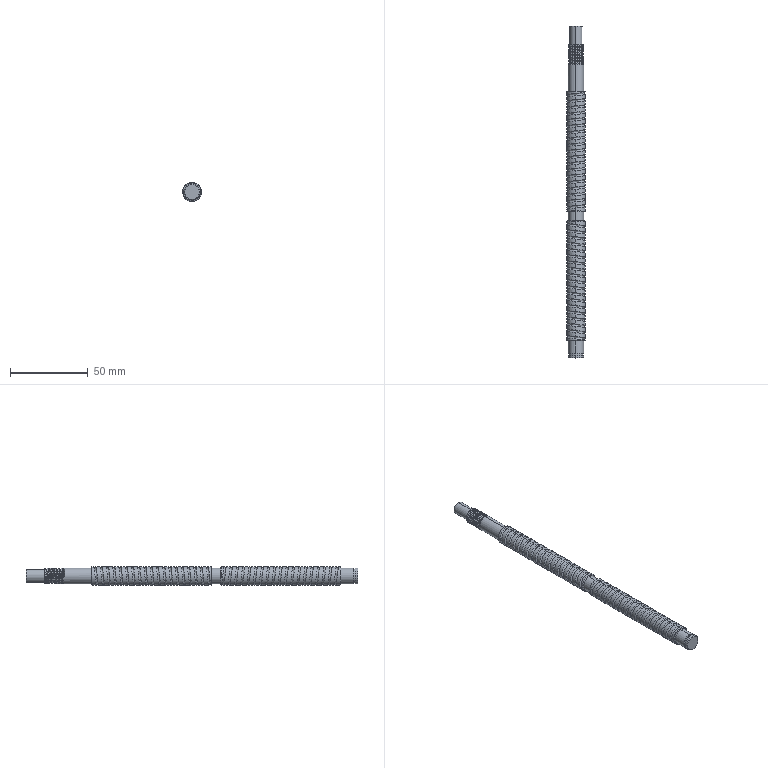Part | SolidWorks | features BaseBody 1 | 1 solid | 148 faces | box 12 x 213 x 12 mm | volume 20380 mm3 | cylinder 116 | cone 14 | plane 13 | spline 5 | commonest cylinder face diameters 12 x80 10 x32 8 x2 9.4 x2